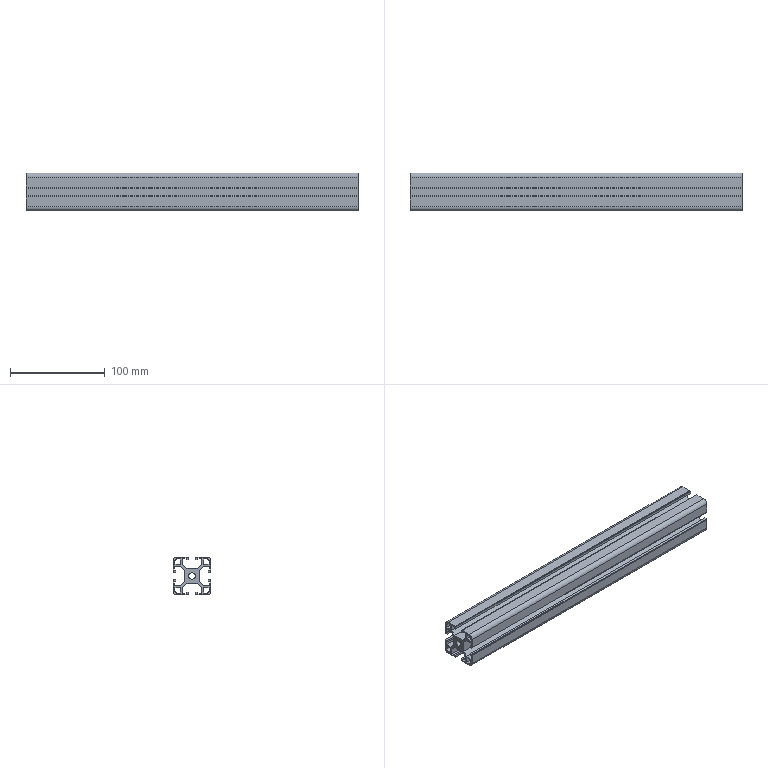Part | SolidWorks | features WeldMemberFeat 1, WeldmentFeature 1 | 1 solid | 104 faces | box 350 x 40 x 40 mm | volume 201791 mm3 | plane 94 | cylinder 10 | commonest cylinder face diameters 5 x4 9 x4 6.8 x2